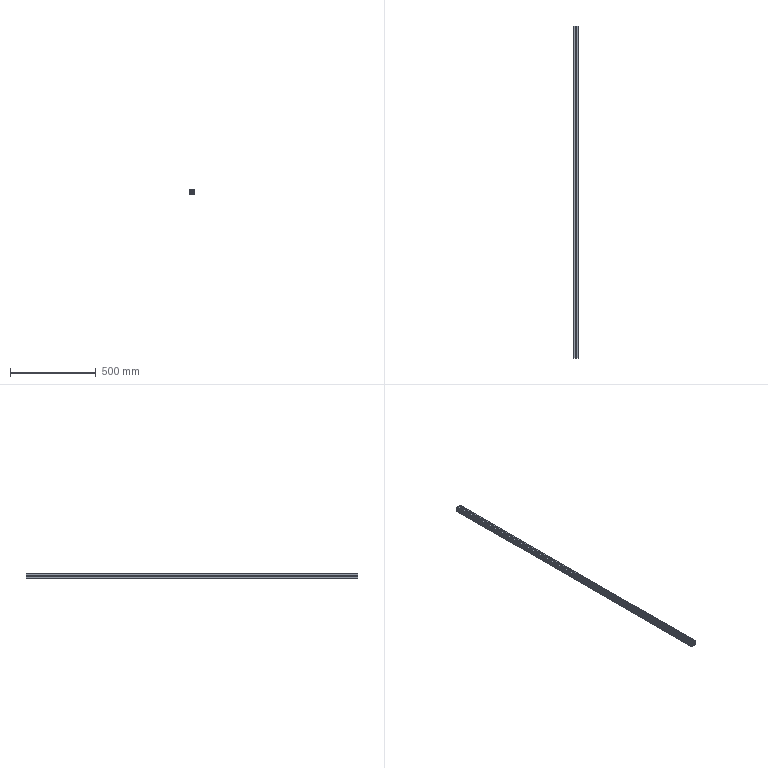Part | SolidWorks | features Extrusion 1 | 1 solid | 60 faces | box 30 x 1940 x 30 mm | volume 645123 mm3 | plane 46 | cylinder 14 | commonest cylinder face diameters 4.2 x8 4 x4 6.8 x2